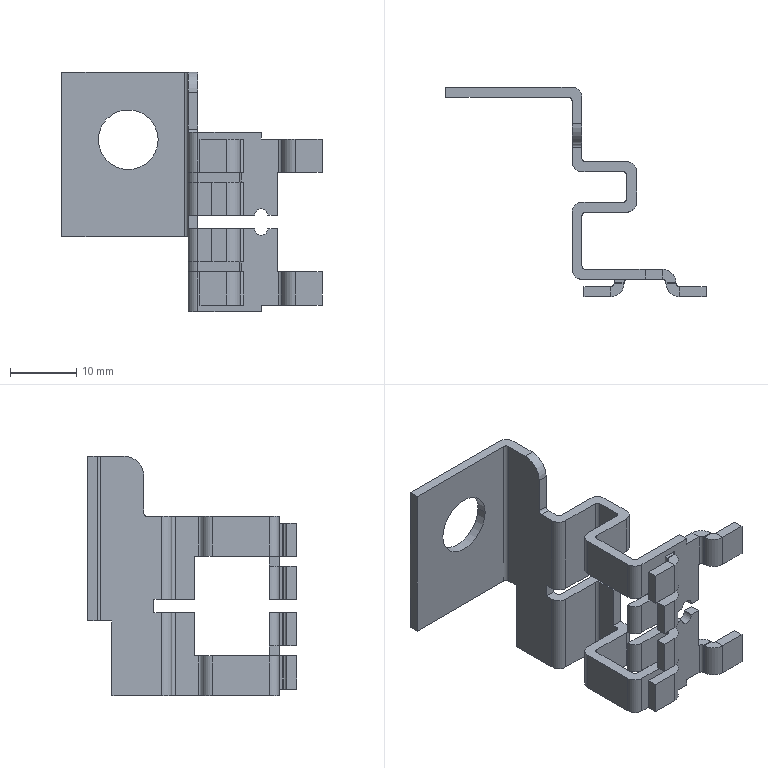Part | SolidWorks | features ICE 10, Fillet 4, FlatPattern 1, LPattern 1, SMBaseFlange 1, SheetMetal 1 | 1 solid | 164 faces | box 39.2 x 31.5 x 36.05 mm | volume 2657 mm3 | plane 110 | cylinder 54 | commonest cylinder face diameters 1 x24 3 x13 4 x12 2 x2 9 x2 6 x1